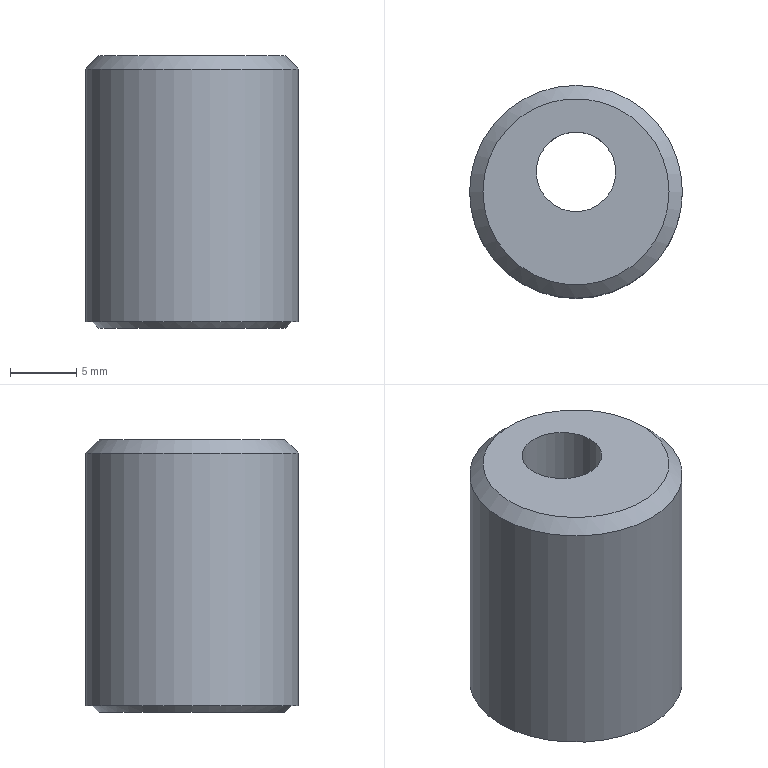Part | NX | features solid 2 | 1 solid | 16 faces | box 16 x 16 x 20.5 mm | volume 3091 mm3 | plane 10 | cylinder 3 | cone 3 | commonest cylinder face diameters 6 x1 9 x1 16 x1
STEP:
#1=CARTESIAN_POINT('',(-297.5,22.,-5.364));
#2=VERTEX_POINT('',#1);
#3=CARTESIAN_POINT('',(-305.,22.,-5.364));
#4=DIRECTION('',(0.,0.,1.));
#5=DIRECTION('',(1.,0.,0.));
#6=AXIS2_PLACEMENT_3D('',#3,#4,#5);
#7=CIRCLE('',#6,7.5);
#8=EDGE_CURVE('',#2,#2,#7,.T.);
#9=ORIENTED_EDGE('',*,*,#8,.T.);
#10=EDGE_LOOP('',(#9));
#11=FACE_BOUND('',#10,.T.);
#12=CARTESIAN_POINT('',(-297.,22.,-5.364));
#13=VERTEX_POINT('',#12);
#14=CARTESIAN_POINT('',(-305.,22.,-5.364));
#15=DIRECTION('',(0.,0.,1.));
#16=DIRECTION('',(1.,0.,0.));
#17=AXIS2_PLACEMENT_3D('',#14,#15,#16);
#18=CIRCLE('',#17,8.);
#19=EDGE_CURVE('',#13,#13,#18,.T.);
#20=ORIENTED_EDGE('',*,*,#19,.F.);
#21=EDGE_LOOP('',(#20));
#22=FACE_BOUND('',#21,.T.);
#23=CARTESIAN_POINT('',(-305.,22.,-5.364));
#24=DIRECTION('',(0.,0.,-1.));
#25=DIRECTION('',(1.,0.,0.));
#26=AXIS2_PLACEMENT_3D('',#23,#24,#25);
#27=PLANE('',#26);
#28=ADVANCED_FACE('',(#11,#22),#27,.T.);
#29=CARTESIAN_POINT('',(-297.,22.,13.636));
#30=VERTEX_POINT('',#29);
#31=CARTESIAN_POINT('',(-305.,22.,13.636));
#32=DIRECTION('',(0.,0.,1.));
#33=DIRECTION('',(1.,0.,0.));
#34=AXIS2_PLACEMENT_3D('',#31,#32,#33);
#35=CIRCLE('',#34,8.);
#36=EDGE_CURVE('',#30,#30,#35,.T.);
#37=ORIENTED_EDGE('',*,*,#36,.F.);
#38=EDGE_LOOP('',(#37));
#39=FACE_BOUND('',#38,.T.);
#40=ORIENTED_EDGE('',*,*,#19,.T.);
#41=EDGE_LOOP('',(#40));
#42=FACE_BOUND('',#41,.T.);
#43=CARTESIAN_POINT('',(-305.,22.,-5.364));
#44=DIRECTION('',(0.,0.,1.));
#45=DIRECTION('',(-1.,0.,0.));
#46=AXIS2_PLACEMENT_3D('',#43,#44,#45);
#47=CYLINDRICAL_SURFACE('',#46,8.);
#48=ADVANCED_FACE('',(#39,#42),#47,.T.);
#49=CARTESIAN_POINT('',(-308.094,18.884,-5.364));
#50=VERTEX_POINT('',#49);
#51=CARTESIAN_POINT('',(-305.025,15.593,-5.364));
#52=VERTEX_POINT('',#51);
#53=CARTESIAN_POINT('',(-308.094,18.884,-5.364));
#54=DIRECTION('',(-0.682,0.7314,0.));
#55=VECTOR('',#54,1000.);
#56=LINE('',#53,#55);
#57=EDGE_CURVE('',#50,#52,#56,.F.);
#58=ORIENTED_EDGE('',*,*,#57,.T.);
#59=CARTESIAN_POINT('',(-301.734,18.662,-5.364));
#60=VERTEX_POINT('',#59);
#61=CARTESIAN_POINT('',(-304.659,15.934,-5.364));
#62=DIRECTION('',(-0.7314,-0.682,0.));
#63=VECTOR('',#62,1000.);
#64=LINE('',#61,#63);
#65=EDGE_CURVE('',#52,#60,#64,.F.);
#66=ORIENTED_EDGE('',*,*,#65,.T.);
#67=CARTESIAN_POINT('',(-302.416,19.394,-5.364));
#68=VERTEX_POINT('',#67);
#69=CARTESIAN_POINT('',(-302.075,19.028,-5.364));
#70=DIRECTION('',(0.682,-0.7314,0.));
#71=VECTOR('',#70,1000.);
#72=LINE('',#69,#71);
#73=EDGE_CURVE('',#68,#60,#72,.T.);
#74=ORIENTED_EDGE('',*,*,#73,.F.);
#75=CARTESIAN_POINT('',(-304.975,17.007,-5.364));
#76=VERTEX_POINT('',#75);
#77=CARTESIAN_POINT('',(-305.341,16.666,-5.364));
#78=DIRECTION('',(-0.7314,-0.682,0.));
#79=VECTOR('',#78,1000.);
#80=LINE('',#77,#79);
#81=EDGE_CURVE('',#76,#68,#80,.F.);
#82=ORIENTED_EDGE('',*,*,#81,.F.);
#83=CARTESIAN_POINT('',(-307.362,19.566,-5.364));
#84=VERTEX_POINT('',#83);
#85=CARTESIAN_POINT('',(-307.362,19.566,-5.364));
#86=DIRECTION('',(-0.682,0.7314,0.));
#87=VECTOR('',#86,1000.);
#88=LINE('',#85,#87);
#89=EDGE_CURVE('',#84,#76,#88,.F.);
#90=ORIENTED_EDGE('',*,*,#89,.F.);
#91=CARTESIAN_POINT('',(-307.728,19.225,-5.364));
#92=DIRECTION('',(-0.7314,-0.682,0.));
#93=VECTOR('',#92,1000.);
#94=LINE('',#91,#93);
#95=EDGE_CURVE('',#84,#50,#94,.T.);
#96=ORIENTED_EDGE('',*,*,#95,.T.);
#97=EDGE_LOOP('',(#58,#66,#74,#82,#90,#96));
#98=FACE_BOUND('',#97,.T.);
#99=CARTESIAN_POINT('',(-298.5,22.,-5.364));
#100=VERTEX_POINT('',#99);
#101=CARTESIAN_POINT('',(-305.,22.,-5.364));
#102=DIRECTION('',(0.,0.,1.));
#103=DIRECTION('',(1.,0.,0.));
#104=AXIS2_PLACEMENT_3D('',#101,#102,#103);
#105=CIRCLE('',#104,6.5);
#106=EDGE_CURVE('',#100,#100,#105,.F.);
#107=ORIENTED_EDGE('',*,*,#106,.T.);
#108=EDGE_LOOP('',(#107));
#109=FACE_BOUND('',#108,.T.);
#110=CARTESIAN_POINT('',(-309.5,23.5,-5.364));
#111=VERTEX_POINT('',#110);
#112=CARTESIAN_POINT('',(-305.,23.5,-5.364));
#113=DIRECTION('',(0.,0.,-1.));
#114=DIRECTION('',(-1.,0.,0.));
#115=AXIS2_PLACEMENT_3D('',#112,#113,#114);
#116=CIRCLE('',#115,4.5);
#117=EDGE_CURVE('',#111,#111,#116,.T.);
#118=ORIENTED_EDGE('',*,*,#117,.F.);
#119=EDGE_LOOP('',(#118));
#120=FACE_BOUND('',#119,.T.);
#121=CARTESIAN_POINT('',(-305.,22.,-5.364));
#122=DIRECTION('',(0.,0.,-1.));
#123=DIRECTION('',(1.,0.,0.));
#124=AXIS2_PLACEMENT_3D('',#121,#122,#123);
#125=PLANE('',#124);
#126=ADVANCED_FACE('',(#98,#109,#120),#125,.T.);
#127=CARTESIAN_POINT('',(-302.,23.5,14.636));
#128=VERTEX_POINT('',#127);
#129=CARTESIAN_POINT('',(-305.,23.5,14.636));
#130=DIRECTION('',(0.,0.,1.));
#131=DIRECTION('',(1.,0.,0.));
#132=AXIS2_PLACEMENT_3D('',#129,#130,#131);
#133=CIRCLE('',#132,3.);
#134=EDGE_CURVE('',#128,#128,#133,.T.);
#135=ORIENTED_EDGE('',*,*,#134,.F.);
#136=EDGE_LOOP('',(#135));
#137=FACE_BOUND('',#136,.T.);
#138=CARTESIAN_POINT('',(-298.,22.,14.636));
#139=VERTEX_POINT('',#138);
#140=CARTESIAN_POINT('',(-305.,22.,14.636));
#141=DIRECTION('',(0.,0.,1.));
#142=DIRECTION('',(1.,0.,0.));
#143=AXIS2_PLACEMENT_3D('',#140,#141,#142);
#144=CIRCLE('',#143,7.);
#145=EDGE_CURVE('',#139,#139,#144,.F.);
#146=ORIENTED_EDGE('',*,*,#145,.F.);
#147=EDGE_LOOP('',(#146));
#148=FACE_BOUND('',#147,.T.);
#149=CARTESIAN_POINT('',(-305.,22.,14.636));
#150=DIRECTION('',(0.,0.,-1.));
#151=DIRECTION('',(1.,0.,0.));
#152=AXIS2_PLACEMENT_3D('',#149,#150,#151);
#153=PLANE('',#152);
#154=ADVANCED_FACE('',(#137,#148),#153,.F.);
#155=ORIENTED_EDGE('',*,*,#145,.T.);
#156=EDGE_LOOP('',(#155));
#157=FACE_BOUND('',#156,.T.);
#158=ORIENTED_EDGE('',*,*,#36,.T.);
#159=EDGE_LOOP('',(#158));
#160=FACE_BOUND('',#159,.T.);
#161=CARTESIAN_POINT('',(-305.,22.,13.636));
#162=DIRECTION('',(0.,0.,-1.));
#163=DIRECTION('',(1.,0.,0.));
#164=AXIS2_PLACEMENT_3D('',#161,#162,#163);
#165=CONICAL_SURFACE('',#164,8.,0.7854);
#166=ADVANCED_FACE('',(#157,#160),#165,.T.);
#167=CARTESIAN_POINT('',(-308.,23.5,4.636));
#168=VERTEX_POINT('',#167);
#169=CARTESIAN_POINT('',(-305.,23.5,4.636));
#170=DIRECTION('',(0.,0.,-1.));
#171=DIRECTION('',(-1.,0.,0.));
#172=AXIS2_PLACEMENT_3D('',#169,#170,#171);
#173=CIRCLE('',#172,3.);
#174=EDGE_CURVE('',#168,#168,#173,.T.);
#175=ORIENTED_EDGE('',*,*,#174,.T.);
#176=EDGE_LOOP('',(#175));
#177=FACE_BOUND('',#176,.T.);
#178=ORIENTED_EDGE('',*,*,#134,.T.);
#179=EDGE_LOOP('',(#178));
#180=FACE_BOUND('',#179,.T.);
#181=CARTESIAN_POINT('',(-305.,23.5,24.636));
#182=DIRECTION('',(0.,0.,1.));
#183=DIRECTION('',(-1.,0.,0.));
#184=AXIS2_PLACEMENT_3D('',#181,#182,#183);
#185=CYLINDRICAL_SURFACE('',#184,3.);
#186=ADVANCED_FACE('',(#177,#180),#185,.F.);
#187=ORIENTED_EDGE('',*,*,#174,.F.);
#188=EDGE_LOOP('',(#187));
#189=FACE_BOUND('',#188,.T.);
#190=CARTESIAN_POINT('',(-309.5,23.5,4.636));
#191=VERTEX_POINT('',#190);
#192=CARTESIAN_POINT('',(-305.,23.5,4.636));
#193=DIRECTION('',(0.,0.,-1.));
#194=DIRECTION('',(-1.,0.,0.));
#195=AXIS2_PLACEMENT_3D('',#192,#193,#194);
#196=CIRCLE('',#195,4.5);
#197=EDGE_CURVE('',#191,#191,#196,.T.);
#198=ORIENTED_EDGE('',*,*,#197,.T.);
#199=EDGE_LOOP('',(#198));
#200=FACE_BOUND('',#199,.T.);
#201=CARTESIAN_POINT('',(-305.,23.5,4.636));
#202=DIRECTION('',(0.,0.,1.));
#203=DIRECTION('',(-1.,0.,0.));
#204=AXIS2_PLACEMENT_3D('',#201,#202,#203);
#205=PLANE('',#204);
#206=ADVANCED_FACE('',(#189,#200),#205,.F.);
#207=ORIENTED_EDGE('',*,*,#197,.F.);
#208=EDGE_LOOP('',(#207));
#209=FACE_BOUND('',#208,.T.);
#210=ORIENTED_EDGE('',*,*,#117,.T.);
#211=EDGE_LOOP('',(#210));
#212=FACE_BOUND('',#211,.T.);
#213=CARTESIAN_POINT('',(-305.,23.5,-5.364));
#214=DIRECTION('',(0.,0.,1.));
#215=DIRECTION('',(-1.,0.,0.));
#216=AXIS2_PLACEMENT_3D('',#213,#214,#215);
#217=CYLINDRICAL_SURFACE('',#216,4.5);
#218=ADVANCED_FACE('',(#209,#212),#217,.F.);
#219=ORIENTED_EDGE('',*,*,#8,.F.);
#220=EDGE_LOOP('',(#219));
#221=FACE_BOUND('',#220,.T.);
#222=CARTESIAN_POINT('',(-312.,22.,-5.864));
#223=VERTEX_POINT('',#222);
#224=CARTESIAN_POINT('',(-305.,22.,-5.864));
#225=DIRECTION('',(0.,0.,-1.));
#226=DIRECTION('',(-1.,0.,0.));
#227=AXIS2_PLACEMENT_3D('',#224,#225,#226);
#228=CIRCLE('',#227,7.);
#229=EDGE_CURVE('',#223,#223,#228,.F.);
#230=ORIENTED_EDGE('',*,*,#229,.T.);
#231=EDGE_LOOP('',(#230));
#232=FACE_BOUND('',#231,.T.);
#233=CARTESIAN_POINT('',(-305.,22.,-5.864));
#234=DIRECTION('',(0.,0.,1.));
#235=DIRECTION('',(-1.,0.,0.));
#236=AXIS2_PLACEMENT_3D('',#233,#234,#235);
#237=CONICAL_SURFACE('',#236,7.,0.7854);
#238=ADVANCED_FACE('',(#221,#232),#237,.T.);
#239=ORIENTED_EDGE('',*,*,#229,.F.);
#240=EDGE_LOOP('',(#239));
#241=FACE_BOUND('',#240,.T.);
#242=ORIENTED_EDGE('',*,*,#106,.F.);
#243=EDGE_LOOP('',(#242));
#244=FACE_BOUND('',#243,.T.);
#245=CARTESIAN_POINT('',(-305.,22.,-5.364));
#246=DIRECTION('',(0.,0.,-1.));
#247=DIRECTION('',(1.,0.,0.));
#248=AXIS2_PLACEMENT_3D('',#245,#246,#247);
#249=CONICAL_SURFACE('',#248,6.5,0.7854);
#250=ADVANCED_FACE('',(#241,#244),#249,.F.);
#251=ORIENTED_EDGE('',*,*,#73,.T.);
#252=CARTESIAN_POINT('',(-302.075,19.028,-5.864));
#253=VERTEX_POINT('',#252);
#254=CARTESIAN_POINT('',(-302.075,19.028,-5.864));
#255=DIRECTION('',(0.4822,-0.5171,0.7071));
#256=VECTOR('',#255,1000.);
#257=LINE('',#254,#256);
#258=EDGE_CURVE('',#253,#60,#257,.T.);
#259=ORIENTED_EDGE('',*,*,#258,.F.);
#260=CARTESIAN_POINT('',(-302.075,19.028,-5.864));
#261=DIRECTION('',(-0.4822,0.5171,0.7071));
#262=VECTOR('',#261,1000.);
#263=LINE('',#260,#262);
#264=EDGE_CURVE('',#68,#253,#263,.F.);
#265=ORIENTED_EDGE('',*,*,#264,.F.);
#266=EDGE_LOOP('',(#251,#259,#265));
#267=FACE_BOUND('',#266,.T.);
#268=CARTESIAN_POINT('',(-302.075,19.028,-5.864));
#269=DIRECTION('',(0.7314,0.682,0.));
#270=DIRECTION('',(0.,0.,1.));
#271=AXIS2_PLACEMENT_3D('',#268,#269,#270);
#272=PLANE('',#271);
#273=ADVANCED_FACE('',(#267),#272,.T.);
#274=CARTESIAN_POINT('',(-307.728,19.225,-5.864));
#275=VERTEX_POINT('',#274);
#276=CARTESIAN_POINT('',(-307.728,19.225,-5.864));
#277=DIRECTION('',(-0.5171,-0.4822,0.7071));
#278=VECTOR('',#277,1000.);
#279=LINE('',#276,#278);
#280=EDGE_CURVE('',#50,#275,#279,.F.);
#281=ORIENTED_EDGE('',*,*,#280,.F.);
#282=ORIENTED_EDGE('',*,*,#95,.F.);
#283=CARTESIAN_POINT('',(-307.728,19.225,-5.864));
#284=DIRECTION('',(0.5171,0.4822,0.7071));
#285=VECTOR('',#284,1000.);
#286=LINE('',#283,#285);
#287=EDGE_CURVE('',#275,#84,#286,.T.);
#288=ORIENTED_EDGE('',*,*,#287,.F.);
#289=EDGE_LOOP('',(#281,#282,#288));
#290=FACE_BOUND('',#289,.T.);
#291=CARTESIAN_POINT('',(-307.728,19.225,-5.864));
#292=DIRECTION('',(0.682,-0.7314,0.));
#293=DIRECTION('',(0.,0.,1.));
#294=AXIS2_PLACEMENT_3D('',#291,#292,#293);
#295=PLANE('',#294);
#296=ADVANCED_FACE('',(#290),#295,.F.);
#297=ORIENTED_EDGE('',*,*,#280,.T.);
#298=CARTESIAN_POINT('',(-305.,16.3,-5.864));
#299=VERTEX_POINT('',#298);
#300=CARTESIAN_POINT('',(-304.659,15.934,-5.864));
#301=DIRECTION('',(0.682,-0.7314,0.));
#302=VECTOR('',#301,1000.);
#303=LINE('',#300,#302);
#304=EDGE_CURVE('',#275,#299,#303,.T.);
#305=ORIENTED_EDGE('',*,*,#304,.T.);
#306=CARTESIAN_POINT('',(-304.934,18.184,-7.197));
#307=DIRECTION('',(0.0285,0.816,-0.5774));
#308=VECTOR('',#307,1000.);
#309=LINE('',#306,#308);
#310=EDGE_CURVE('',#299,#52,#309,.F.);
#311=ORIENTED_EDGE('',*,*,#310,.T.);
#312=ORIENTED_EDGE('',*,*,#57,.F.);
#313=EDGE_LOOP('',(#297,#305,#311,#312));
#314=FACE_BOUND('',#313,.T.);
#315=CARTESIAN_POINT('',(-307.728,19.225,-5.864));
#316=DIRECTION('',(-0.5171,-0.4822,-0.7071));
#317=DIRECTION('',(0.8072,0.,-0.5903));
#318=AXIS2_PLACEMENT_3D('',#315,#316,#317);
#319=PLANE('',#318);
#320=ADVANCED_FACE('',(#314),#319,.T.);
#321=ORIENTED_EDGE('',*,*,#65,.F.);
#322=ORIENTED_EDGE('',*,*,#310,.F.);
#323=CARTESIAN_POINT('',(-302.075,19.028,-5.864));
#324=DIRECTION('',(0.7314,0.682,0.));
#325=VECTOR('',#324,1000.);
#326=LINE('',#323,#325);
#327=EDGE_CURVE('',#299,#253,#326,.T.);
#328=ORIENTED_EDGE('',*,*,#327,.T.);
#329=ORIENTED_EDGE('',*,*,#258,.T.);
#330=EDGE_LOOP('',(#321,#322,#328,#329));
#331=FACE_BOUND('',#330,.T.);
#332=CARTESIAN_POINT('',(-305.,16.3,-5.864));
#333=DIRECTION('',(0.4822,-0.5171,-0.7071));
#334=DIRECTION('',(0.,-0.8072,0.5903));
#335=AXIS2_PLACEMENT_3D('',#332,#333,#334);
#336=PLANE('',#335);
#337=ADVANCED_FACE('',(#331),#336,.T.);
#338=ORIENTED_EDGE('',*,*,#287,.T.);
#339=ORIENTED_EDGE('',*,*,#89,.T.);
#340=CARTESIAN_POINT('',(-304.984,16.771,-5.53));
#341=DIRECTION('',(0.0285,0.816,0.5774));
#342=VECTOR('',#341,1000.);
#343=LINE('',#340,#342);
#344=EDGE_CURVE('',#76,#299,#343,.F.);
#345=ORIENTED_EDGE('',*,*,#344,.T.);
#346=ORIENTED_EDGE('',*,*,#304,.F.);
#347=EDGE_LOOP('',(#338,#339,#345,#346));
#348=FACE_BOUND('',#347,.T.);
#349=CARTESIAN_POINT('',(-307.362,19.566,-5.364));
#350=DIRECTION('',(-0.5171,-0.4822,0.7071));
#351=DIRECTION('',(-0.8072,0.,-0.5903));
#352=AXIS2_PLACEMENT_3D('',#349,#350,#351);
#353=PLANE('',#352);
#354=ADVANCED_FACE('',(#348),#353,.F.);
#355=ORIENTED_EDGE('',*,*,#344,.F.);
#356=ORIENTED_EDGE('',*,*,#81,.T.);
#357=ORIENTED_EDGE('',*,*,#264,.T.);
#358=ORIENTED_EDGE('',*,*,#327,.F.);
#359=EDGE_LOOP('',(#355,#356,#357,#358));
#360=FACE_BOUND('',#359,.T.);
#361=CARTESIAN_POINT('',(-305.341,16.666,-5.364));
#362=DIRECTION('',(0.4822,-0.5171,0.7071));
#363=DIRECTION('',(0.,0.8072,0.5903));
#364=AXIS2_PLACEMENT_3D('',#361,#362,#363);
#365=PLANE('',#364);
#366=ADVANCED_FACE('',(#360),#365,.F.);
#367=CLOSED_SHELL('',(#28,#48,#126,#154,#166,#186,#206,#218,#238,#250,#273,#296,#320,#337,#354,#366));
#368=MANIFOLD_SOLID_BREP('',#367);
#369=(LENGTH_UNIT()NAMED_UNIT(*)SI_UNIT(.MILLI.,.METRE.));
#370=UNCERTAINTY_MEASURE_WITH_UNIT(LENGTH_MEASURE(0.00001),#369,'','');
#371=(NAMED_UNIT(*)PLANE_ANGLE_UNIT()SI_UNIT($,.RADIAN.));
#372=(NAMED_UNIT(*)SI_UNIT($,.STERADIAN.)SOLID_ANGLE_UNIT());
#373=(GEOMETRIC_REPRESENTATION_CONTEXT(3)GLOBAL_UNCERTAINTY_ASSIGNED_CONTEXT((#370))GLOBAL_UNIT_ASSIGNED_CONTEXT((#369,#371,#372))REPRESENTATION_CONTEXT('',''));
#374=ADVANCED_BREP_SHAPE_REPRESENTATION('',(#368),#373);